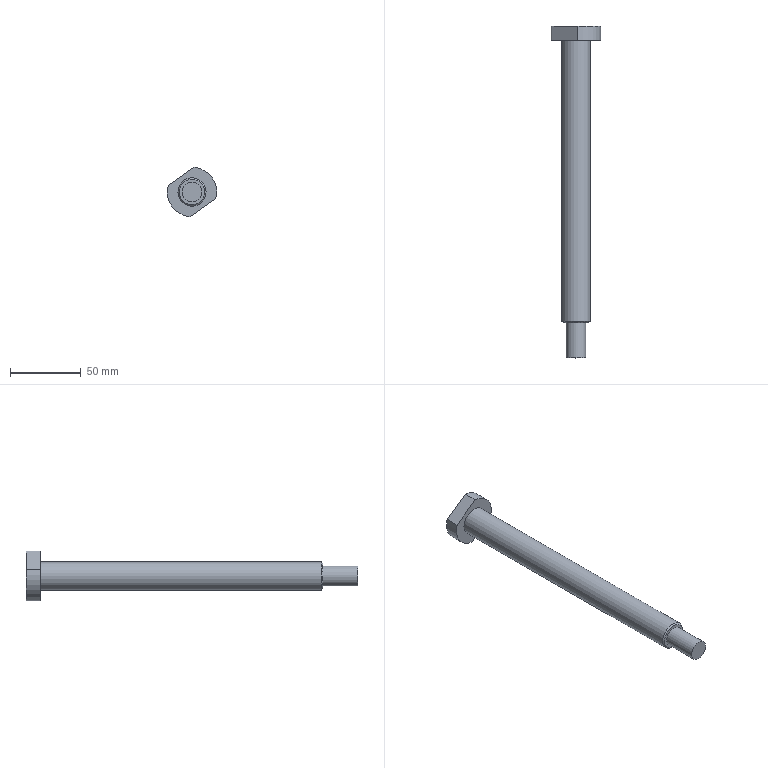Part | STEP file | HL4GZ-1.862.041 (cane-lifter mechanism mounting pin weldment) | 2 solids | 15 faces | box 35 x 235 x 34.891 mm | volume 74372 mm3 | plane 8 | cylinder 6 | cone 1 | commonest cylinder face diameters 17 x2 35 x2 14 x1 20 x1
STEP:
#1=CARTESIAN_POINT('',(0.,0.,0.));
#2=DIRECTION('',(0.,0.,1.));
#3=DIRECTION('',(1.,0.,0.));
#4=AXIS2_PLACEMENT_3D('',#1,#2,#3);
#5=CARTESIAN_POINT('',(3183.622,700.,-296.446));
#6=VERTEX_POINT('',#5);
#7=CARTESIAN_POINT('',(3183.622,690.,-296.446));
#8=VERTEX_POINT('',#7);
#9=CARTESIAN_POINT('',(3183.622,698.,-296.446));
#10=DIRECTION('',(0.,-1.,0.));
#11=VECTOR('',#10,1.);
#12=LINE('',#9,#11);
#13=CARTESIAN_POINT('',(3192.743,691.5,-290.059));
#14=DIRECTION('',(0.5736,0.,-0.8192));
#15=DIRECTION('',(0.8192,0.,0.5736));
#16=AXIS2_PLACEMENT_3D('',#13,#14,#15);
#17=PLANE('',#16);
#18=CARTESIAN_POINT('',(-11.136,-6.5));
#19=DIRECTION('',(0.,1.));
#20=VECTOR('',#19,1.);
#21=LINE('',#18,#20);
#22=(GEOMETRIC_REPRESENTATION_CONTEXT(2)PARAMETRIC_REPRESENTATION_CONTEXT()REPRESENTATION_CONTEXT('',''));
#23=DEFINITIONAL_REPRESENTATION('',(#21),#22);
#24=PCURVE('',#17,#23);
#25=CARTESIAN_POINT('',(3185.,690.,-279.));
#26=DIRECTION('',(0.,1.,0.));
#27=DIRECTION('',(0.06875,0.,0.9976));
#28=AXIS2_PLACEMENT_3D('',#25,#26,#27);
#29=CYLINDRICAL_SURFACE('',#28,17.5);
#30=CARTESIAN_POINT('',(3.152,8.));
#31=DIRECTION('',(0.,-1.));
#32=VECTOR('',#31,1.);
#33=LINE('',#30,#32);
#34=(GEOMETRIC_REPRESENTATION_CONTEXT(2)PARAMETRIC_REPRESENTATION_CONTEXT()REPRESENTATION_CONTEXT('',''));
#35=DEFINITIONAL_REPRESENTATION('',(#33),#34);
#36=PCURVE('',#29,#35);
#37=SURFACE_CURVE('',#12,(#24,#36),.PCURVE_S1.);
#38=EDGE_CURVE('',#6,#8,#37,.T.);
#39=ORIENTED_EDGE('',*,*,#38,.F.);
#40=CARTESIAN_POINT('',(3201.865,700.,-283.671));
#41=VERTEX_POINT('',#40);
#42=CARTESIAN_POINT('',(3192.743,700.,-290.059));
#43=DIRECTION('',(0.8192,0.,0.5736));
#44=VECTOR('',#43,1.);
#45=LINE('',#42,#44);
#46=CARTESIAN_POINT('',(0.,-8.5));
#47=DIRECTION('',(1.,0.));
#48=VECTOR('',#47,1.);
#49=LINE('',#46,#48);
#50=(GEOMETRIC_REPRESENTATION_CONTEXT(2)PARAMETRIC_REPRESENTATION_CONTEXT()REPRESENTATION_CONTEXT('',''));
#51=DEFINITIONAL_REPRESENTATION('',(#49),#50);
#52=PCURVE('',#17,#51);
#53=CARTESIAN_POINT('',(3184.927,700.,-278.896));
#54=DIRECTION('',(0.,-1.,0.));
#55=DIRECTION('',(0.8192,0.,0.5736));
#56=AXIS2_PLACEMENT_3D('',#53,#54,#55);
#57=PLANE('',#56);
#58=CARTESIAN_POINT('',(0.,-13.627));
#59=DIRECTION('',(1.,0.));
#60=VECTOR('',#59,1.);
#61=LINE('',#58,#60);
#62=(GEOMETRIC_REPRESENTATION_CONTEXT(2)PARAMETRIC_REPRESENTATION_CONTEXT()REPRESENTATION_CONTEXT('',''));
#63=DEFINITIONAL_REPRESENTATION('',(#61),#62);
#64=PCURVE('',#57,#63);
#65=SURFACE_CURVE('',#45,(#52,#64),.PCURVE_S1.);
#66=EDGE_CURVE('',#6,#41,#65,.T.);
#67=ORIENTED_EDGE('',*,*,#66,.T.);
#68=CARTESIAN_POINT('',(3201.865,690.,-283.671));
#69=VERTEX_POINT('',#68);
#70=CARTESIAN_POINT('',(3201.865,690.,-283.671));
#71=DIRECTION('',(0.,1.,0.));
#72=VECTOR('',#71,1.);
#73=LINE('',#70,#72);
#74=CARTESIAN_POINT('',(11.136,1.5));
#75=DIRECTION('',(0.,-1.));
#76=VECTOR('',#75,1.);
#77=LINE('',#74,#76);
#78=(GEOMETRIC_REPRESENTATION_CONTEXT(2)PARAMETRIC_REPRESENTATION_CONTEXT()REPRESENTATION_CONTEXT('',''));
#79=DEFINITIONAL_REPRESENTATION('',(#77),#78);
#80=PCURVE('',#17,#79);
#81=CARTESIAN_POINT('',(3185.,690.,-279.));
#82=DIRECTION('',(0.,1.,0.));
#83=DIRECTION('',(0.06875,0.,0.9976));
#84=AXIS2_PLACEMENT_3D('',#81,#82,#83);
#85=CYLINDRICAL_SURFACE('',#84,17.5);
#86=CARTESIAN_POINT('',(1.772,0.));
#87=DIRECTION('',(0.,1.));
#88=VECTOR('',#87,1.);
#89=LINE('',#86,#88);
#90=(GEOMETRIC_REPRESENTATION_CONTEXT(2)PARAMETRIC_REPRESENTATION_CONTEXT()REPRESENTATION_CONTEXT('',''));
#91=DEFINITIONAL_REPRESENTATION('',(#89),#90);
#92=PCURVE('',#85,#91);
#93=SURFACE_CURVE('',#73,(#80,#92),.PCURVE_S1.);
#94=EDGE_CURVE('',#69,#41,#93,.T.);
#95=ORIENTED_EDGE('',*,*,#94,.F.);
#96=CARTESIAN_POINT('',(3192.743,690.,-290.059));
#97=DIRECTION('',(0.8192,0.,0.5736));
#98=VECTOR('',#97,1.);
#99=LINE('',#96,#98);
#100=CARTESIAN_POINT('',(0.,1.5));
#101=DIRECTION('',(1.,0.));
#102=VECTOR('',#101,1.);
#103=LINE('',#100,#102);
#104=(GEOMETRIC_REPRESENTATION_CONTEXT(2)PARAMETRIC_REPRESENTATION_CONTEXT()REPRESENTATION_CONTEXT('',''));
#105=DEFINITIONAL_REPRESENTATION('',(#103),#104);
#106=PCURVE('',#17,#105);
#107=CARTESIAN_POINT('',(3184.927,690.,-278.896));
#108=DIRECTION('',(0.,-1.,0.));
#109=DIRECTION('',(0.8192,0.,0.5736));
#110=AXIS2_PLACEMENT_3D('',#107,#108,#109);
#111=PLANE('',#110);
#112=CARTESIAN_POINT('',(0.,-13.627));
#113=DIRECTION('',(1.,0.));
#114=VECTOR('',#113,1.);
#115=LINE('',#112,#114);
#116=(GEOMETRIC_REPRESENTATION_CONTEXT(2)PARAMETRIC_REPRESENTATION_CONTEXT()REPRESENTATION_CONTEXT('',''));
#117=DEFINITIONAL_REPRESENTATION('',(#115),#116);
#118=PCURVE('',#111,#117);
#119=SURFACE_CURVE('',#99,(#106,#118),.PCURVE_S1.);
#120=EDGE_CURVE('',#8,#69,#119,.T.);
#121=ORIENTED_EDGE('',*,*,#120,.F.);
#122=EDGE_LOOP('',(#39,#67,#95,#121));
#123=FACE_BOUND('',#122,.T.);
#124=ADVANCED_FACE('',(#123),#17,.T.);
#125=CARTESIAN_POINT('',(3168.135,690.,-274.328));
#126=VERTEX_POINT('',#125);
#127=CARTESIAN_POINT('',(3186.378,690.,-261.554));
#128=VERTEX_POINT('',#127);
#129=CARTESIAN_POINT('',(3167.989,690.,-274.431));
#130=DIRECTION('',(0.8192,0.,0.5736));
#131=VECTOR('',#130,1.);
#132=LINE('',#129,#131);
#133=CARTESIAN_POINT('',(3167.989,690.,-274.431));
#134=DIRECTION('',(-0.5736,0.,0.8192));
#135=DIRECTION('',(0.8192,0.,0.5736));
#136=AXIS2_PLACEMENT_3D('',#133,#134,#135);
#137=PLANE('',#136);
#138=CARTESIAN_POINT('',(0.,0.));
#139=DIRECTION('',(1.,0.));
#140=VECTOR('',#139,1.);
#141=LINE('',#138,#140);
#142=(GEOMETRIC_REPRESENTATION_CONTEXT(2)PARAMETRIC_REPRESENTATION_CONTEXT()REPRESENTATION_CONTEXT('',''));
#143=DEFINITIONAL_REPRESENTATION('',(#141),#142);
#144=PCURVE('',#137,#143);
#145=CARTESIAN_POINT('',(-11.314,13.373));
#146=DIRECTION('',(1.,0.));
#147=VECTOR('',#146,1.);
#148=LINE('',#145,#147);
#149=(GEOMETRIC_REPRESENTATION_CONTEXT(2)PARAMETRIC_REPRESENTATION_CONTEXT()REPRESENTATION_CONTEXT('',''));
#150=DEFINITIONAL_REPRESENTATION('',(#148),#149);
#151=PCURVE('',#111,#150);
#152=SURFACE_CURVE('',#132,(#144,#151),.PCURVE_S1.);
#153=EDGE_CURVE('',#126,#128,#152,.T.);
#154=ORIENTED_EDGE('',*,*,#153,.T.);
#155=CARTESIAN_POINT('',(3186.378,700.,-261.554));
#156=VERTEX_POINT('',#155);
#157=CARTESIAN_POINT('',(3186.378,690.,-261.554));
#158=DIRECTION('',(0.,1.,0.));
#159=VECTOR('',#158,1.);
#160=LINE('',#157,#159);
#161=CARTESIAN_POINT('',(22.449,0.));
#162=DIRECTION('',(0.,1.));
#163=VECTOR('',#162,1.);
#164=LINE('',#161,#163);
#165=(GEOMETRIC_REPRESENTATION_CONTEXT(2)PARAMETRIC_REPRESENTATION_CONTEXT()REPRESENTATION_CONTEXT('',''));
#166=DEFINITIONAL_REPRESENTATION('',(#164),#165);
#167=PCURVE('',#137,#166);
#168=CARTESIAN_POINT('',(0.01004,0.));
#169=DIRECTION('',(0.,1.));
#170=VECTOR('',#169,1.);
#171=LINE('',#168,#170);
#172=(GEOMETRIC_REPRESENTATION_CONTEXT(2)PARAMETRIC_REPRESENTATION_CONTEXT()REPRESENTATION_CONTEXT('',''));
#173=DEFINITIONAL_REPRESENTATION('',(#171),#172);
#174=PCURVE('',#85,#173);
#175=SURFACE_CURVE('',#160,(#167,#174),.PCURVE_S1.);
#176=EDGE_CURVE('',#128,#156,#175,.T.);
#177=ORIENTED_EDGE('',*,*,#176,.T.);
#178=CARTESIAN_POINT('',(3168.135,700.,-274.328));
#179=VERTEX_POINT('',#178);
#180=CARTESIAN_POINT('',(3167.989,700.,-274.431));
#181=DIRECTION('',(0.8192,0.,0.5736));
#182=VECTOR('',#181,1.);
#183=LINE('',#180,#182);
#184=CARTESIAN_POINT('',(0.,10.));
#185=DIRECTION('',(1.,0.));
#186=VECTOR('',#185,1.);
#187=LINE('',#184,#186);
#188=(GEOMETRIC_REPRESENTATION_CONTEXT(2)PARAMETRIC_REPRESENTATION_CONTEXT()REPRESENTATION_CONTEXT('',''));
#189=DEFINITIONAL_REPRESENTATION('',(#187),#188);
#190=PCURVE('',#137,#189);
#191=CARTESIAN_POINT('',(-11.314,13.373));
#192=DIRECTION('',(1.,0.));
#193=VECTOR('',#192,1.);
#194=LINE('',#191,#193);
#195=(GEOMETRIC_REPRESENTATION_CONTEXT(2)PARAMETRIC_REPRESENTATION_CONTEXT()REPRESENTATION_CONTEXT('',''));
#196=DEFINITIONAL_REPRESENTATION('',(#194),#195);
#197=PCURVE('',#57,#196);
#198=SURFACE_CURVE('',#183,(#190,#197),.PCURVE_S1.);
#199=EDGE_CURVE('',#179,#156,#198,.T.);
#200=ORIENTED_EDGE('',*,*,#199,.F.);
#201=CARTESIAN_POINT('',(3168.135,690.,-274.328));
#202=DIRECTION('',(0.,1.,0.));
#203=VECTOR('',#202,1.);
#204=LINE('',#201,#203);
#205=CARTESIAN_POINT('',(0.1782,0.));
#206=DIRECTION('',(0.,1.));
#207=VECTOR('',#206,1.);
#208=LINE('',#205,#207);
#209=(GEOMETRIC_REPRESENTATION_CONTEXT(2)PARAMETRIC_REPRESENTATION_CONTEXT()REPRESENTATION_CONTEXT('',''));
#210=DEFINITIONAL_REPRESENTATION('',(#208),#209);
#211=PCURVE('',#137,#210);
#212=CARTESIAN_POINT('',(4.914,0.));
#213=DIRECTION('',(0.,1.));
#214=VECTOR('',#213,1.);
#215=LINE('',#212,#214);
#216=(GEOMETRIC_REPRESENTATION_CONTEXT(2)PARAMETRIC_REPRESENTATION_CONTEXT()REPRESENTATION_CONTEXT('',''));
#217=DEFINITIONAL_REPRESENTATION('',(#215),#216);
#218=PCURVE('',#29,#217);
#219=SURFACE_CURVE('',#204,(#211,#218),.PCURVE_S1.);
#220=EDGE_CURVE('',#126,#179,#219,.T.);
#221=ORIENTED_EDGE('',*,*,#220,.F.);
#222=EDGE_LOOP('',(#154,#177,#200,#221));
#223=FACE_BOUND('',#222,.T.);
#224=ADVANCED_FACE('',(#223),#137,.T.);
#225=CARTESIAN_POINT('',(3185.,690.,-287.5));
#226=VERTEX_POINT('',#225);
#227=CARTESIAN_POINT('',(3185.,690.,-279.));
#228=DIRECTION('',(0.,1.,0.));
#229=DIRECTION('',(0.,0.,-1.));
#230=AXIS2_PLACEMENT_3D('',#227,#228,#229);
#231=CIRCLE('',#230,8.5);
#232=CARTESIAN_POINT('',(3185.,690.,-279.));
#233=DIRECTION('',(0.,1.,0.));
#234=DIRECTION('',(0.8192,0.,0.5736));
#235=AXIS2_PLACEMENT_3D('',#232,#233,#234);
#236=CYLINDRICAL_SURFACE('',#235,8.5);
#237=CARTESIAN_POINT('',(2.182,0.));
#238=DIRECTION('',(1.,0.));
#239=VECTOR('',#238,1.);
#240=LINE('',#237,#239);
#241=(GEOMETRIC_REPRESENTATION_CONTEXT(2)PARAMETRIC_REPRESENTATION_CONTEXT()REPRESENTATION_CONTEXT('',''));
#242=DEFINITIONAL_REPRESENTATION('',(#240),#241);
#243=PCURVE('',#236,#242);
#244=CARTESIAN_POINT('',(-4.875,-7.09));
#245=CARTESIAN_POINT('',(-16.935,1.355));
#246=CARTESIAN_POINT('',(-3.592,7.577));
#247=CARTESIAN_POINT('',(9.751,13.799));
#248=CARTESIAN_POINT('',(8.468,-0.8678));
#249=CARTESIAN_POINT('',(7.185,-15.534));
#250=CARTESIAN_POINT('',(-4.875,-7.09));
#251=(BOUNDED_CURVE()B_SPLINE_CURVE(2,(#244,#245,#246,#247,#248,#249,#250),.UNSPECIFIED.,.T.,.F.)B_SPLINE_CURVE_WITH_KNOTS((1,2,2,2,2,1),(-2.094,0.,2.094,4.189,6.283,8.378),.UNSPECIFIED.)CURVE()GEOMETRIC_REPRESENTATION_ITEM()RATIONAL_B_SPLINE_CURVE((1.,0.5,1.,0.5,1.,0.5,1.))REPRESENTATION_ITEM(''));
#252=(GEOMETRIC_REPRESENTATION_CONTEXT(2)PARAMETRIC_REPRESENTATION_CONTEXT()REPRESENTATION_CONTEXT('',''));
#253=DEFINITIONAL_REPRESENTATION('',(#251),#252);
#254=PCURVE('',#111,#253);
#255=SURFACE_CURVE('',#231,(#243,#254),.PCURVE_S1.);
#256=EDGE_CURVE('',#226,#226,#255,.T.);
#257=ORIENTED_EDGE('',*,*,#256,.T.);
#258=CARTESIAN_POINT('',(3185.,700.,-287.5));
#259=VERTEX_POINT('',#258);
#260=CARTESIAN_POINT('',(3185.,690.,-287.5));
#261=CARTESIAN_POINT('',(3185.,700.,-287.5));
#262=B_SPLINE_CURVE_WITH_KNOTS('',1,(#260,#261),.UNSPECIFIED.,.F.,.F.,(2,2),(0.,10.),.PIECEWISE_BEZIER_KNOTS.);
#263=CARTESIAN_POINT('',(8.465,0.));
#264=DIRECTION('',(0.,1.));
#265=VECTOR('',#264,1.);
#266=LINE('',#263,#265);
#267=(GEOMETRIC_REPRESENTATION_CONTEXT(2)PARAMETRIC_REPRESENTATION_CONTEXT()REPRESENTATION_CONTEXT('',''));
#268=DEFINITIONAL_REPRESENTATION('',(#266),#267);
#269=PCURVE('',#236,#268);
#270=CARTESIAN_POINT('',(2.182,0.));
#271=DIRECTION('',(0.,1.));
#272=VECTOR('',#271,1.);
#273=LINE('',#270,#272);
#274=(GEOMETRIC_REPRESENTATION_CONTEXT(2)PARAMETRIC_REPRESENTATION_CONTEXT()REPRESENTATION_CONTEXT('',''));
#275=DEFINITIONAL_REPRESENTATION('',(#273),#274);
#276=PCURVE('',#236,#275);
#277=SEAM_CURVE('',#262,(#269,#276),.PCURVE_S1.);
#278=EDGE_CURVE('',#226,#259,#277,.T.);
#279=ORIENTED_EDGE('',*,*,#278,.T.);
#280=CARTESIAN_POINT('',(3185.,700.,-279.));
#281=DIRECTION('',(0.,-1.,0.));
#282=DIRECTION('',(0.,0.,-1.));
#283=AXIS2_PLACEMENT_3D('',#280,#281,#282);
#284=CIRCLE('',#283,8.5);
#285=CARTESIAN_POINT('',(8.465,10.));
#286=DIRECTION('',(-1.,0.));
#287=VECTOR('',#286,1.);
#288=LINE('',#285,#287);
#289=(GEOMETRIC_REPRESENTATION_CONTEXT(2)PARAMETRIC_REPRESENTATION_CONTEXT()REPRESENTATION_CONTEXT('',''));
#290=DEFINITIONAL_REPRESENTATION('',(#288),#289);
#291=PCURVE('',#236,#290);
#292=CARTESIAN_POINT('',(0.,-0.127));
#293=DIRECTION('',(-0.5736,-0.8192));
#294=AXIS2_PLACEMENT_2D('',#292,#293);
#295=CIRCLE('',#294,8.5);
#296=(GEOMETRIC_REPRESENTATION_CONTEXT(2)PARAMETRIC_REPRESENTATION_CONTEXT()REPRESENTATION_CONTEXT('',''));
#297=DEFINITIONAL_REPRESENTATION('',(#295),#296);
#298=PCURVE('',#57,#297);
#299=SURFACE_CURVE('',#284,(#291,#298),.PCURVE_S1.);
#300=EDGE_CURVE('',#259,#259,#299,.T.);
#301=ORIENTED_EDGE('',*,*,#300,.T.);
#302=ORIENTED_EDGE('',*,*,#278,.F.);
#303=EDGE_LOOP('',(#257,#279,#301,#302));
#304=FACE_BOUND('',#303,.F.);
#305=ADVANCED_FACE('',(#304),#236,.F.);
#306=CARTESIAN_POINT('',(3185.,690.,-279.));
#307=DIRECTION('',(0.,1.,0.));
#308=DIRECTION('',(0.,0.,-1.));
#309=AXIS2_PLACEMENT_3D('',#306,#307,#308);
#310=CIRCLE('',#309,17.5);
#311=CARTESIAN_POINT('',(-10.038,-14.462));
#312=CARTESIAN_POINT('',(-34.867,2.923));
#313=CARTESIAN_POINT('',(-7.396,15.733));
#314=CARTESIAN_POINT('',(20.075,28.543));
#315=CARTESIAN_POINT('',(17.433,-1.652));
#316=CARTESIAN_POINT('',(14.792,-31.848));
#317=CARTESIAN_POINT('',(-10.038,-14.462));
#318=(BOUNDED_CURVE()B_SPLINE_CURVE(2,(#311,#312,#313,#314,#315,#316,#317),.UNSPECIFIED.,.T.,.F.)B_SPLINE_CURVE_WITH_KNOTS((1,2,2,2,2,1),(-2.094,0.,2.094,4.189,6.283,8.378),.UNSPECIFIED.)CURVE()GEOMETRIC_REPRESENTATION_ITEM()RATIONAL_B_SPLINE_CURVE((1.,0.5,1.,0.5,1.,0.5,1.))REPRESENTATION_ITEM(''));
#319=(GEOMETRIC_REPRESENTATION_CONTEXT(2)PARAMETRIC_REPRESENTATION_CONTEXT()REPRESENTATION_CONTEXT('',''));
#320=DEFINITIONAL_REPRESENTATION('',(#318),#319);
#321=PCURVE('',#111,#320);
#322=CARTESIAN_POINT('',(3.073,0.));
#323=DIRECTION('',(1.,0.));
#324=VECTOR('',#323,1.);
#325=LINE('',#322,#324);
#326=(GEOMETRIC_REPRESENTATION_CONTEXT(2)PARAMETRIC_REPRESENTATION_CONTEXT()REPRESENTATION_CONTEXT('',''));
#327=DEFINITIONAL_REPRESENTATION('',(#325),#326);
#328=PCURVE('',#29,#327);
#329=SURFACE_CURVE('',#310,(#321,#328),.PCURVE_S1.);
#330=EDGE_CURVE('',#8,#126,#329,.T.);
#331=ORIENTED_EDGE('',*,*,#330,.F.);
#332=ORIENTED_EDGE('',*,*,#120,.T.);
#333=CARTESIAN_POINT('',(3185.,690.,-279.));
#334=DIRECTION('',(0.,1.,0.));
#335=DIRECTION('',(0.,0.,-1.));
#336=AXIS2_PLACEMENT_3D('',#333,#334,#335);
#337=CIRCLE('',#336,17.5);
#338=CARTESIAN_POINT('',(-10.038,-14.462));
#339=CARTESIAN_POINT('',(-34.867,2.923));
#340=CARTESIAN_POINT('',(-7.396,15.733));
#341=CARTESIAN_POINT('',(20.075,28.543));
#342=CARTESIAN_POINT('',(17.433,-1.652));
#343=CARTESIAN_POINT('',(14.792,-31.848));
#344=CARTESIAN_POINT('',(-10.038,-14.462));
#345=(BOUNDED_CURVE()B_SPLINE_CURVE(2,(#338,#339,#340,#341,#342,#343,#344),.UNSPECIFIED.,.T.,.F.)B_SPLINE_CURVE_WITH_KNOTS((1,2,2,2,2,1),(-2.094,0.,2.094,4.189,6.283,8.378),.UNSPECIFIED.)CURVE()GEOMETRIC_REPRESENTATION_ITEM()RATIONAL_B_SPLINE_CURVE((1.,0.5,1.,0.5,1.,0.5,1.))REPRESENTATION_ITEM(''));
#346=(GEOMETRIC_REPRESENTATION_CONTEXT(2)PARAMETRIC_REPRESENTATION_CONTEXT()REPRESENTATION_CONTEXT('',''));
#347=DEFINITIONAL_REPRESENTATION('',(#345),#346);
#348=PCURVE('',#111,#347);
#349=CARTESIAN_POINT('',(-3.21,0.));
#350=DIRECTION('',(1.,0.));
#351=VECTOR('',#350,1.);
#352=LINE('',#349,#351);
#353=(GEOMETRIC_REPRESENTATION_CONTEXT(2)PARAMETRIC_REPRESENTATION_CONTEXT()REPRESENTATION_CONTEXT('',''));
#354=DEFINITIONAL_REPRESENTATION('',(#352),#353);
#355=PCURVE('',#85,#354);
#356=SURFACE_CURVE('',#337,(#348,#355),.PCURVE_S1.);
#357=EDGE_CURVE('',#128,#69,#356,.T.);
#358=ORIENTED_EDGE('',*,*,#357,.F.);
#359=ORIENTED_EDGE('',*,*,#153,.F.);
#360=EDGE_LOOP('',(#331,#332,#358,#359));
#361=FACE_BOUND('',#360,.T.);
#362=ORIENTED_EDGE('',*,*,#256,.T.);
#363=EDGE_LOOP('',(#362));
#364=FACE_BOUND('',#363,.T.);
#365=ADVANCED_FACE('',(#361,#364),#111,.T.);
#366=ORIENTED_EDGE('',*,*,#66,.F.);
#367=CARTESIAN_POINT('',(3185.,700.,-279.));
#368=DIRECTION('',(0.,1.,0.));
#369=DIRECTION('',(0.,0.,-1.));
#370=AXIS2_PLACEMENT_3D('',#367,#368,#369);
#371=CIRCLE('',#370,17.5);
#372=CARTESIAN_POINT('',(-10.038,-14.462));
#373=CARTESIAN_POINT('',(-34.867,2.923));
#374=CARTESIAN_POINT('',(-7.396,15.733));
#375=CARTESIAN_POINT('',(20.075,28.543));
#376=CARTESIAN_POINT('',(17.433,-1.652));
#377=CARTESIAN_POINT('',(14.792,-31.848));
#378=CARTESIAN_POINT('',(-10.038,-14.462));
#379=(BOUNDED_CURVE()B_SPLINE_CURVE(2,(#372,#373,#374,#375,#376,#377,#378),.UNSPECIFIED.,.T.,.F.)B_SPLINE_CURVE_WITH_KNOTS((1,2,2,2,2,1),(-2.094,0.,2.094,4.189,6.283,8.378),.UNSPECIFIED.)CURVE()GEOMETRIC_REPRESENTATION_ITEM()RATIONAL_B_SPLINE_CURVE((1.,0.5,1.,0.5,1.,0.5,1.))REPRESENTATION_ITEM(''));
#380=(GEOMETRIC_REPRESENTATION_CONTEXT(2)PARAMETRIC_REPRESENTATION_CONTEXT()REPRESENTATION_CONTEXT('',''));
#381=DEFINITIONAL_REPRESENTATION('',(#379),#380);
#382=PCURVE('',#57,#381);
#383=CARTESIAN_POINT('',(3.073,10.));
#384=DIRECTION('',(1.,0.));
#385=VECTOR('',#384,1.);
#386=LINE('',#383,#385);
#387=(GEOMETRIC_REPRESENTATION_CONTEXT(2)PARAMETRIC_REPRESENTATION_CONTEXT()REPRESENTATION_CONTEXT('',''));
#388=DEFINITIONAL_REPRESENTATION('',(#386),#387);
#389=PCURVE('',#29,#388);
#390=SURFACE_CURVE('',#371,(#382,#389),.PCURVE_S1.);
#391=EDGE_CURVE('',#6,#179,#390,.T.);
#392=ORIENTED_EDGE('',*,*,#391,.T.);
#393=ORIENTED_EDGE('',*,*,#199,.T.);
#394=CARTESIAN_POINT('',(3185.,700.,-279.));
#395=DIRECTION('',(0.,1.,0.));
#396=DIRECTION('',(0.,0.,-1.));
#397=AXIS2_PLACEMENT_3D('',#394,#395,#396);
#398=CIRCLE('',#397,17.5);
#399=CARTESIAN_POINT('',(-10.038,-14.462));
#400=CARTESIAN_POINT('',(-34.867,2.923));
#401=CARTESIAN_POINT('',(-7.396,15.733));
#402=CARTESIAN_POINT('',(20.075,28.543));
#403=CARTESIAN_POINT('',(17.433,-1.652));
#404=CARTESIAN_POINT('',(14.792,-31.848));
#405=CARTESIAN_POINT('',(-10.038,-14.462));
#406=(BOUNDED_CURVE()B_SPLINE_CURVE(2,(#399,#400,#401,#402,#403,#404,#405),.UNSPECIFIED.,.T.,.F.)B_SPLINE_CURVE_WITH_KNOTS((1,2,2,2,2,1),(-2.094,0.,2.094,4.189,6.283,8.378),.UNSPECIFIED.)CURVE()GEOMETRIC_REPRESENTATION_ITEM()RATIONAL_B_SPLINE_CURVE((1.,0.5,1.,0.5,1.,0.5,1.))REPRESENTATION_ITEM(''));
#407=(GEOMETRIC_REPRESENTATION_CONTEXT(2)PARAMETRIC_REPRESENTATION_CONTEXT()REPRESENTATION_CONTEXT('',''));
#408=DEFINITIONAL_REPRESENTATION('',(#406),#407);
#409=PCURVE('',#57,#408);
#410=CARTESIAN_POINT('',(-3.21,10.));
#411=DIRECTION('',(1.,0.));
#412=VECTOR('',#411,1.);
#413=LINE('',#410,#412);
#414=(GEOMETRIC_REPRESENTATION_CONTEXT(2)PARAMETRIC_REPRESENTATION_CONTEXT()REPRESENTATION_CONTEXT('',''));
#415=DEFINITIONAL_REPRESENTATION('',(#413),#414);
#416=PCURVE('',#85,#415);
#417=SURFACE_CURVE('',#398,(#409,#416),.PCURVE_S1.);
#418=EDGE_CURVE('',#156,#41,#417,.T.);
#419=ORIENTED_EDGE('',*,*,#418,.T.);
#420=EDGE_LOOP('',(#366,#392,#393,#419));
#421=FACE_BOUND('',#420,.T.);
#422=ORIENTED_EDGE('',*,*,#300,.T.);
#423=EDGE_LOOP('',(#422));
#424=FACE_BOUND('',#423,.T.);
#425=ADVANCED_FACE('',(#421,#424),#57,.F.);
#426=ORIENTED_EDGE('',*,*,#357,.T.);
#427=ORIENTED_EDGE('',*,*,#94,.T.);
#428=ORIENTED_EDGE('',*,*,#418,.F.);
#429=ORIENTED_EDGE('',*,*,#176,.F.);
#430=EDGE_LOOP('',(#426,#427,#428,#429));
#431=FACE_BOUND('',#430,.T.);
#432=ADVANCED_FACE('',(#431),#85,.T.);
#433=ORIENTED_EDGE('',*,*,#391,.F.);
#434=ORIENTED_EDGE('',*,*,#38,.T.);
#435=ORIENTED_EDGE('',*,*,#330,.T.);
#436=ORIENTED_EDGE('',*,*,#220,.T.);
#437=EDGE_LOOP('',(#433,#434,#435,#436));
#438=FACE_BOUND('',#437,.T.);
#439=ADVANCED_FACE('',(#438),#29,.T.);
#440=CLOSED_SHELL('',(#124,#224,#305,#365,#425,#432,#439));
#441=MANIFOLD_SOLID_BREP('',#440);
#442=CARTESIAN_POINT('',(3185.,490.,-286.));
#443=VERTEX_POINT('',#442);
#444=CARTESIAN_POINT('',(3185.,490.,-279.));
#445=DIRECTION('',(0.,-1.,0.));
#446=DIRECTION('',(0.,0.,-1.));
#447=AXIS2_PLACEMENT_3D('',#444,#445,#446);
#448=CIRCLE('',#447,7.);
#449=CARTESIAN_POINT('',(3185.,477.,-279.));
#450=DIRECTION('',(0.,-1.,0.));
#451=DIRECTION('',(0.5736,0.,-0.8192));
#452=AXIS2_PLACEMENT_3D('',#449,#450,#451);
#453=CYLINDRICAL_SURFACE('',#452,7.);
#454=CARTESIAN_POINT('',(5.672,-13.));
#455=DIRECTION('',(1.,0.));
#456=VECTOR('',#455,1.);
#457=LINE('',#454,#456);
#458=(GEOMETRIC_REPRESENTATION_CONTEXT(2)PARAMETRIC_REPRESENTATION_CONTEXT()REPRESENTATION_CONTEXT('',''));
#459=DEFINITIONAL_REPRESENTATION('',(#457),#458);
#460=PCURVE('',#453,#459);
#461=CARTESIAN_POINT('',(3188.441,490.,-283.915));
#462=DIRECTION('',(0.,-1.,0.));
#463=DIRECTION('',(-0.8192,0.,-0.5736));
#464=AXIS2_PLACEMENT_3D('',#461,#462,#463);
#465=PLANE('',#464);
#466=CARTESIAN_POINT('',(0.,-6.));
#467=DIRECTION('',(0.5736,0.8192));
#468=AXIS2_PLACEMENT_2D('',#466,#467);
#469=CIRCLE('',#468,7.);
#470=(GEOMETRIC_REPRESENTATION_CONTEXT(2)PARAMETRIC_REPRESENTATION_CONTEXT()REPRESENTATION_CONTEXT('',''));
#471=DEFINITIONAL_REPRESENTATION('',(#469),#470);
#472=PCURVE('',#465,#471);
#473=SURFACE_CURVE('',#448,(#460,#472),.PCURVE_S1.);
#474=EDGE_CURVE('',#443,#443,#473,.T.);
#475=ORIENTED_EDGE('',*,*,#474,.T.);
#476=CARTESIAN_POINT('',(3185.,465.,-286.));
#477=VERTEX_POINT('',#476);
#478=CARTESIAN_POINT('',(3185.,490.,-286.));
#479=CARTESIAN_POINT('',(3185.,465.,-286.));
#480=B_SPLINE_CURVE_WITH_KNOTS('',1,(#478,#479),.UNSPECIFIED.,.F.,.F.,(2,2),(-13.,12.),.PIECEWISE_BEZIER_KNOTS.);
#481=CARTESIAN_POINT('',(11.956,0.));
#482=DIRECTION('',(0.,1.));
#483=VECTOR('',#482,1.);
#484=LINE('',#481,#483);
#485=(GEOMETRIC_REPRESENTATION_CONTEXT(2)PARAMETRIC_REPRESENTATION_CONTEXT()REPRESENTATION_CONTEXT('',''));
#486=DEFINITIONAL_REPRESENTATION('',(#484),#485);
#487=PCURVE('',#453,#486);
#488=CARTESIAN_POINT('',(5.672,0.));
#489=DIRECTION('',(0.,1.));
#490=VECTOR('',#489,1.);
#491=LINE('',#488,#490);
#492=(GEOMETRIC_REPRESENTATION_CONTEXT(2)PARAMETRIC_REPRESENTATION_CONTEXT()REPRESENTATION_CONTEXT('',''));
#493=DEFINITIONAL_REPRESENTATION('',(#491),#492);
#494=PCURVE('',#453,#493);
#495=SEAM_CURVE('',#480,(#487,#494),.PCURVE_S1.);
#496=EDGE_CURVE('',#443,#477,#495,.T.);
#497=ORIENTED_EDGE('',*,*,#496,.T.);
#498=CARTESIAN_POINT('',(3185.,465.,-279.));
#499=DIRECTION('',(0.,-1.,0.));
#500=DIRECTION('',(0.,0.,-1.));
#501=AXIS2_PLACEMENT_3D('',#498,#499,#500);
#502=CIRCLE('',#501,7.);
#503=CARTESIAN_POINT('',(5.672,12.));
#504=DIRECTION('',(1.,0.));
#505=VECTOR('',#504,1.);
#506=LINE('',#503,#505);
#507=(GEOMETRIC_REPRESENTATION_CONTEXT(2)PARAMETRIC_REPRESENTATION_CONTEXT()REPRESENTATION_CONTEXT('',''));
#508=DEFINITIONAL_REPRESENTATION('',(#506),#507);
#509=PCURVE('',#453,#508);
#510=CARTESIAN_POINT('',(3185.,465.,-279.));
#511=DIRECTION('',(0.,-1.,0.));
#512=DIRECTION('',(-0.8192,0.,-0.5736));
#513=AXIS2_PLACEMENT_3D('',#510,#511,#512);
#514=PLANE('',#513);
#515=CARTESIAN_POINT('',(0.,0.));
#516=DIRECTION('',(0.5736,0.8192));
#517=AXIS2_PLACEMENT_2D('',#515,#516);
#518=CIRCLE('',#517,7.);
#519=(GEOMETRIC_REPRESENTATION_CONTEXT(2)PARAMETRIC_REPRESENTATION_CONTEXT()REPRESENTATION_CONTEXT('',''));
#520=DEFINITIONAL_REPRESENTATION('',(#518),#519);
#521=PCURVE('',#514,#520);
#522=SURFACE_CURVE('',#502,(#509,#521),.PCURVE_S1.);
#523=EDGE_CURVE('',#477,#477,#522,.T.);
#524=ORIENTED_EDGE('',*,*,#523,.F.);
#525=ORIENTED_EDGE('',*,*,#496,.F.);
#526=EDGE_LOOP('',(#475,#497,#524,#525));
#527=FACE_BOUND('',#526,.T.);
#528=ADVANCED_FACE('',(#527),#453,.T.);
#529=CARTESIAN_POINT('',(3185.,690.,-270.5));
#530=VERTEX_POINT('',#529);
#531=CARTESIAN_POINT('',(3185.,690.,-287.5));
#532=VERTEX_POINT('',#531);
#533=CARTESIAN_POINT('',(3185.,690.,-279.));
#534=DIRECTION('',(0.,-1.,0.));
#535=DIRECTION('',(0.,0.,1.));
#536=AXIS2_PLACEMENT_3D('',#533,#534,#535);
#537=CIRCLE('',#536,8.5);
#538=CARTESIAN_POINT('',(3190.736,690.,-287.191));
#539=DIRECTION('',(0.,1.,0.));
#540=DIRECTION('',(0.8192,0.,0.5736));
#541=AXIS2_PLACEMENT_3D('',#538,#539,#540);
#542=PLANE('',#541);
#543=CARTESIAN_POINT('',(4.875,-16.963));
#544=CARTESIAN_POINT('',(-7.185,-25.407));
#545=CARTESIAN_POINT('',(-8.468,-10.741));
#546=CARTESIAN_POINT('',(-9.751,3.926));
#547=CARTESIAN_POINT('',(3.592,-2.296));
#548=CARTESIAN_POINT('',(16.935,-8.518));
#549=CARTESIAN_POINT('',(4.875,-16.963));
#550=(BOUNDED_CURVE()B_SPLINE_CURVE(2,(#543,#544,#545,#546,#547,#548,#549),.UNSPECIFIED.,.T.,.F.)B_SPLINE_CURVE_WITH_KNOTS((1,2,2,2,2,1),(-2.094,0.,2.094,4.189,6.283,8.378),.UNSPECIFIED.)CURVE()GEOMETRIC_REPRESENTATION_ITEM()RATIONAL_B_SPLINE_CURVE((1.,0.5,1.,0.5,1.,0.5,1.))REPRESENTATION_ITEM(''));
#551=(GEOMETRIC_REPRESENTATION_CONTEXT(2)PARAMETRIC_REPRESENTATION_CONTEXT()REPRESENTATION_CONTEXT('',''));
#552=DEFINITIONAL_REPRESENTATION('',(#550),#551);
#553=PCURVE('',#542,#552);
#554=CARTESIAN_POINT('',(3185.,690.,-279.));
#555=DIRECTION('',(0.,1.,0.));
#556=DIRECTION('',(-0.8192,0.,-0.5736));
#557=AXIS2_PLACEMENT_3D('',#554,#555,#556);
#558=CYLINDRICAL_SURFACE('',#557,8.5);
#559=CARTESIAN_POINT('',(8.465,0.));
#560=DIRECTION('',(-1.,0.));
#561=VECTOR('',#560,1.);
#562=LINE('',#559,#561);
#563=(GEOMETRIC_REPRESENTATION_CONTEXT(2)PARAMETRIC_REPRESENTATION_CONTEXT()REPRESENTATION_CONTEXT('',''));
#564=DEFINITIONAL_REPRESENTATION('',(#562),#563);
#565=PCURVE('',#558,#564);
#566=SURFACE_CURVE('',#537,(#553,#565),.PCURVE_S1.);
#567=EDGE_CURVE('',#530,#532,#566,.T.);
#568=ORIENTED_EDGE('',*,*,#567,.T.);
#569=CARTESIAN_POINT('',(3185.,690.,-279.));
#570=DIRECTION('',(0.,-1.,0.));
#571=DIRECTION('',(0.,0.,1.));
#572=AXIS2_PLACEMENT_3D('',#569,#570,#571);
#573=CIRCLE('',#572,8.5);
#574=CARTESIAN_POINT('',(4.875,-16.963));
#575=CARTESIAN_POINT('',(-7.185,-25.407));
#576=CARTESIAN_POINT('',(-8.468,-10.741));
#577=CARTESIAN_POINT('',(-9.751,3.926));
#578=CARTESIAN_POINT('',(3.592,-2.296));
#579=CARTESIAN_POINT('',(16.935,-8.518));
#580=CARTESIAN_POINT('',(4.875,-16.963));
#581=(BOUNDED_CURVE()B_SPLINE_CURVE(2,(#574,#575,#576,#577,#578,#579,#580),.UNSPECIFIED.,.T.,.F.)B_SPLINE_CURVE_WITH_KNOTS((1,2,2,2,2,1),(-2.094,0.,2.094,4.189,6.283,8.378),.UNSPECIFIED.)CURVE()GEOMETRIC_REPRESENTATION_ITEM()RATIONAL_B_SPLINE_CURVE((1.,0.5,1.,0.5,1.,0.5,1.))REPRESENTATION_ITEM(''));
#582=(GEOMETRIC_REPRESENTATION_CONTEXT(2)PARAMETRIC_REPRESENTATION_CONTEXT()REPRESENTATION_CONTEXT('',''));
#583=DEFINITIONAL_REPRESENTATION('',(#581),#582);
#584=PCURVE('',#542,#583);
#585=CARTESIAN_POINT('',(14.748,0.));
#586=DIRECTION('',(-1.,0.));
#587=VECTOR('',#586,1.);
#588=LINE('',#585,#587);
#589=(GEOMETRIC_REPRESENTATION_CONTEXT(2)PARAMETRIC_REPRESENTATION_CONTEXT()REPRESENTATION_CONTEXT('',''));
#590=DEFINITIONAL_REPRESENTATION('',(#588),#589);
#591=PCURVE('',#558,#590);
#592=SURFACE_CURVE('',#573,(#584,#591),.PCURVE_S1.);
#593=EDGE_CURVE('',#532,#530,#592,.T.);
#594=ORIENTED_EDGE('',*,*,#593,.T.);
#595=EDGE_LOOP('',(#568,#594));
#596=FACE_BOUND('',#595,.T.);
#597=CARTESIAN_POINT('',(3190.736,690.,-287.191));
#598=VERTEX_POINT('',#597);
#599=CARTESIAN_POINT('',(3185.,690.,-279.));
#600=DIRECTION('',(0.,-1.,0.));
#601=DIRECTION('',(-0.8192,0.,-0.5736));
#602=AXIS2_PLACEMENT_3D('',#599,#600,#601);
#603=CIRCLE('',#602,10.);
#604=CARTESIAN_POINT('',(-10.,-10.));
#605=CARTESIAN_POINT('',(-10.,7.321));
#606=CARTESIAN_POINT('',(5.,-1.34));
#607=CARTESIAN_POINT('',(20.,-10.));
#608=CARTESIAN_POINT('',(5.,-18.66));
#609=CARTESIAN_POINT('',(-10.,-27.321));
#610=CARTESIAN_POINT('',(-10.,-10.));
#611=(BOUNDED_CURVE()B_SPLINE_CURVE(2,(#604,#605,#606,#607,#608,#609,#610),.UNSPECIFIED.,.T.,.F.)B_SPLINE_CURVE_WITH_KNOTS((1,2,2,2,2,1),(-2.094,0.,2.094,4.189,6.283,8.378),.UNSPECIFIED.)CURVE()GEOMETRIC_REPRESENTATION_ITEM()RATIONAL_B_SPLINE_CURVE((1.,0.5,1.,0.5,1.,0.5,1.))REPRESENTATION_ITEM(''));
#612=(GEOMETRIC_REPRESENTATION_CONTEXT(2)PARAMETRIC_REPRESENTATION_CONTEXT()REPRESENTATION_CONTEXT('',''));
#613=DEFINITIONAL_REPRESENTATION('',(#611),#612);
#614=PCURVE('',#542,#613);
#615=CARTESIAN_POINT('',(3185.,590.,-279.));
#616=DIRECTION('',(0.,-1.,0.));
#617=DIRECTION('',(0.5736,0.,-0.8192));
#618=AXIS2_PLACEMENT_3D('',#615,#616,#617);
#619=CYLINDRICAL_SURFACE('',#618,10.);
#620=CARTESIAN_POINT('',(-1.571,-100.));
#621=DIRECTION('',(1.,0.));
#622=VECTOR('',#621,1.);
#623=LINE('',#620,#622);
#624=(GEOMETRIC_REPRESENTATION_CONTEXT(2)PARAMETRIC_REPRESENTATION_CONTEXT()REPRESENTATION_CONTEXT('',''));
#625=DEFINITIONAL_REPRESENTATION('',(#623),#624);
#626=PCURVE('',#619,#625);
#627=SURFACE_CURVE('',#603,(#614,#626),.PCURVE_S1.);
#628=EDGE_CURVE('',#598,#598,#627,.T.);
#629=ORIENTED_EDGE('',*,*,#628,.F.);
#630=EDGE_LOOP('',(#629));
#631=FACE_BOUND('',#630,.T.);
#632=ADVANCED_FACE('',(#596,#631),#542,.T.);
#633=CARTESIAN_POINT('',(3185.,697.,-287.5));
#634=VERTEX_POINT('',#633);
#635=CARTESIAN_POINT('',(3185.,697.,-279.));
#636=DIRECTION('',(0.,1.,0.));
#637=DIRECTION('',(0.,0.,-1.));
#638=AXIS2_PLACEMENT_3D('',#635,#636,#637);
#639=CIRCLE('',#638,8.5);
#640=CARTESIAN_POINT('',(3185.,697.,-279.));
#641=DIRECTION('',(0.,-1.,0.));
#642=DIRECTION('',(-0.8192,0.,-0.5736));
#643=AXIS2_PLACEMENT_3D('',#640,#641,#642);
#644=PLANE('',#643);
#645=CARTESIAN_POINT('',(4.875,6.963));
#646=CARTESIAN_POINT('',(16.935,-1.482));
#647=CARTESIAN_POINT('',(3.592,-7.704));
#648=CARTESIAN_POINT('',(-9.751,-13.926));
#649=CARTESIAN_POINT('',(-8.468,0.7408));
#650=CARTESIAN_POINT('',(-7.185,15.407));
#651=CARTESIAN_POINT('',(4.875,6.963));
#652=(BOUNDED_CURVE()B_SPLINE_CURVE(2,(#645,#646,#647,#648,#649,#650,#651),.UNSPECIFIED.,.T.,.F.)B_SPLINE_CURVE_WITH_KNOTS((1,2,2,2,2,1),(-2.094,0.,2.094,4.189,6.283,8.378),.UNSPECIFIED.)CURVE()GEOMETRIC_REPRESENTATION_ITEM()RATIONAL_B_SPLINE_CURVE((1.,0.5,1.,0.5,1.,0.5,1.))REPRESENTATION_ITEM(''));
#653=(GEOMETRIC_REPRESENTATION_CONTEXT(2)PARAMETRIC_REPRESENTATION_CONTEXT()REPRESENTATION_CONTEXT('',''));
#654=DEFINITIONAL_REPRESENTATION('',(#652),#653);
#655=PCURVE('',#644,#654);
#656=CARTESIAN_POINT('',(5.323,7.));
#657=DIRECTION('',(1.,0.));
#658=VECTOR('',#657,1.);
#659=LINE('',#656,#658);
#660=(GEOMETRIC_REPRESENTATION_CONTEXT(2)PARAMETRIC_REPRESENTATION_CONTEXT()REPRESENTATION_CONTEXT('',''));
#661=DEFINITIONAL_REPRESENTATION('',(#659),#660);
#662=PCURVE('',#558,#661);
#663=SURFACE_CURVE('',#639,(#655,#662),.PCURVE_S1.);
#664=EDGE_CURVE('',#634,#634,#663,.T.);
#665=ORIENTED_EDGE('',*,*,#664,.T.);
#666=EDGE_LOOP('',(#665));
#667=FACE_BOUND('',#666,.T.);
#668=ADVANCED_FACE('',(#667),#644,.F.);
#669=ORIENTED_EDGE('',*,*,#593,.F.);
#670=CARTESIAN_POINT('',(3185.,690.,-287.5));
#671=CARTESIAN_POINT('',(3185.,697.,-287.5));
#672=B_SPLINE_CURVE_WITH_KNOTS('',1,(#670,#671),.UNSPECIFIED.,.F.,.F.,(2,2),(0.,7.),.PIECEWISE_BEZIER_KNOTS.);
#673=CARTESIAN_POINT('',(11.606,0.));
#674=DIRECTION('',(0.,1.));
#675=VECTOR('',#674,1.);
#676=LINE('',#673,#675);
#677=(GEOMETRIC_REPRESENTATION_CONTEXT(2)PARAMETRIC_REPRESENTATION_CONTEXT()REPRESENTATION_CONTEXT('',''));
#678=DEFINITIONAL_REPRESENTATION('',(#676),#677);
#679=PCURVE('',#558,#678);
#680=CARTESIAN_POINT('',(5.323,0.));
#681=DIRECTION('',(0.,1.));
#682=VECTOR('',#681,1.);
#683=LINE('',#680,#682);
#684=(GEOMETRIC_REPRESENTATION_CONTEXT(2)PARAMETRIC_REPRESENTATION_CONTEXT()REPRESENTATION_CONTEXT('',''));
#685=DEFINITIONAL_REPRESENTATION('',(#683),#684);
#686=PCURVE('',#558,#685);
#687=SEAM_CURVE('',#672,(#679,#686),.PCURVE_S1.);
#688=EDGE_CURVE('',#532,#634,#687,.T.);
#689=ORIENTED_EDGE('',*,*,#688,.T.);
#690=ORIENTED_EDGE('',*,*,#664,.F.);
#691=ORIENTED_EDGE('',*,*,#688,.F.);
#692=ORIENTED_EDGE('',*,*,#567,.F.);
#693=EDGE_LOOP('',(#669,#689,#690,#691,#692));
#694=FACE_BOUND('',#693,.T.);
#695=ADVANCED_FACE('',(#694),#558,.T.);
#696=CARTESIAN_POINT('',(3190.162,490.,-286.372));
#697=VERTEX_POINT('',#696);
#698=CARTESIAN_POINT('',(3185.,490.,-279.));
#699=DIRECTION('',(0.,1.,0.));
#700=DIRECTION('',(-0.5736,0.,0.8192));
#701=AXIS2_PLACEMENT_3D('',#698,#699,#700);
#702=CIRCLE('',#701,9.);
#703=CARTESIAN_POINT('',(0.,-15.));
#704=CARTESIAN_POINT('',(-15.588,-15.));
#705=CARTESIAN_POINT('',(-7.794,-1.5));
#706=CARTESIAN_POINT('',(0.,12.));
#707=CARTESIAN_POINT('',(7.794,-1.5));
#708=CARTESIAN_POINT('',(15.588,-15.));
#709=CARTESIAN_POINT('',(0.,-15.));
#710=(BOUNDED_CURVE()B_SPLINE_CURVE(2,(#703,#704,#705,#706,#707,#708,#709),.UNSPECIFIED.,.T.,.F.)B_SPLINE_CURVE_WITH_KNOTS((1,2,2,2,2,1),(-2.094,0.,2.094,4.189,6.283,8.378),.UNSPECIFIED.)CURVE()GEOMETRIC_REPRESENTATION_ITEM()RATIONAL_B_SPLINE_CURVE((1.,0.5,1.,0.5,1.,0.5,1.))REPRESENTATION_ITEM(''));
#711=(GEOMETRIC_REPRESENTATION_CONTEXT(2)PARAMETRIC_REPRESENTATION_CONTEXT()REPRESENTATION_CONTEXT('',''));
#712=DEFINITIONAL_REPRESENTATION('',(#710),#711);
#713=PCURVE('',#465,#712);
#714=CARTESIAN_POINT('',(3185.,490.5,-279.));
#715=DIRECTION('',(0.,1.,0.));
#716=DIRECTION('',(-0.5736,0.,0.8192));
#717=AXIS2_PLACEMENT_3D('',#714,#715,#716);
#718=CONICAL_SURFACE('',#717,9.5,0.7854);
#719=CARTESIAN_POINT('',(0.,-0.5));
#720=DIRECTION('',(1.,0.));
#721=VECTOR('',#720,1.);
#722=LINE('',#719,#721);
#723=(GEOMETRIC_REPRESENTATION_CONTEXT(2)PARAMETRIC_REPRESENTATION_CONTEXT()REPRESENTATION_CONTEXT('',''));
#724=DEFINITIONAL_REPRESENTATION('',(#722),#723);
#725=PCURVE('',#718,#724);
#726=SURFACE_CURVE('',#702,(#713,#725),.PCURVE_S1.);
#727=EDGE_CURVE('',#697,#697,#726,.T.);
#728=ORIENTED_EDGE('',*,*,#727,.F.);
#729=EDGE_LOOP('',(#728));
#730=FACE_BOUND('',#729,.T.);
#731=ORIENTED_EDGE('',*,*,#474,.F.);
#732=EDGE_LOOP('',(#731));
#733=FACE_BOUND('',#732,.T.);
#734=ADVANCED_FACE('',(#730,#733),#465,.T.);
#735=CARTESIAN_POINT('',(3190.736,491.,-287.191));
#736=VERTEX_POINT('',#735);
#737=CARTESIAN_POINT('',(3185.,491.,-279.));
#738=DIRECTION('',(0.,-1.,0.));
#739=DIRECTION('',(-0.5736,0.,0.8192));
#740=AXIS2_PLACEMENT_3D('',#737,#738,#739);
#741=CIRCLE('',#740,10.);
#742=CARTESIAN_POINT('',(-3.142,99.));
#743=DIRECTION('',(1.,0.));
#744=VECTOR('',#743,1.);
#745=LINE('',#742,#744);
#746=(GEOMETRIC_REPRESENTATION_CONTEXT(2)PARAMETRIC_REPRESENTATION_CONTEXT()REPRESENTATION_CONTEXT('',''));
#747=DEFINITIONAL_REPRESENTATION('',(#745),#746);
#748=PCURVE('',#619,#747);
#749=CARTESIAN_POINT('',(12.566,0.5));
#750=DIRECTION('',(-1.,0.));
#751=VECTOR('',#750,1.);
#752=LINE('',#749,#751);
#753=(GEOMETRIC_REPRESENTATION_CONTEXT(2)PARAMETRIC_REPRESENTATION_CONTEXT()REPRESENTATION_CONTEXT('',''));
#754=DEFINITIONAL_REPRESENTATION('',(#752),#753);
#755=PCURVE('',#718,#754);
#756=SURFACE_CURVE('',#741,(#748,#755),.PCURVE_S1.);
#757=EDGE_CURVE('',#736,#736,#756,.T.);
#758=ORIENTED_EDGE('',*,*,#757,.F.);
#759=CARTESIAN_POINT('',(3190.736,690.,-287.191));
#760=CARTESIAN_POINT('',(3190.736,491.,-287.191));
#761=B_SPLINE_CURVE_WITH_KNOTS('',1,(#759,#760),.UNSPECIFIED.,.F.,.F.,(2,2),(-100.,99.),.PIECEWISE_BEZIER_KNOTS.);
#762=CARTESIAN_POINT('',(0.,0.));
#763=DIRECTION('',(0.,1.));
#764=VECTOR('',#763,1.);
#765=LINE('',#762,#764);
#766=(GEOMETRIC_REPRESENTATION_CONTEXT(2)PARAMETRIC_REPRESENTATION_CONTEXT()REPRESENTATION_CONTEXT('',''));
#767=DEFINITIONAL_REPRESENTATION('',(#765),#766);
#768=PCURVE('',#619,#767);
#769=CARTESIAN_POINT('',(6.283,0.));
#770=DIRECTION('',(0.,1.));
#771=VECTOR('',#770,1.);
#772=LINE('',#769,#771);
#773=(GEOMETRIC_REPRESENTATION_CONTEXT(2)PARAMETRIC_REPRESENTATION_CONTEXT()REPRESENTATION_CONTEXT('',''));
#774=DEFINITIONAL_REPRESENTATION('',(#772),#773);
#775=PCURVE('',#619,#774);
#776=SEAM_CURVE('',#761,(#768,#775),.PCURVE_S1.);
#777=EDGE_CURVE('',#598,#736,#776,.T.);
#778=ORIENTED_EDGE('',*,*,#777,.F.);
#779=ORIENTED_EDGE('',*,*,#628,.T.);
#780=ORIENTED_EDGE('',*,*,#777,.T.);
#781=EDGE_LOOP('',(#758,#778,#779,#780));
#782=FACE_BOUND('',#781,.T.);
#783=ADVANCED_FACE('',(#782),#619,.T.);
#784=ORIENTED_EDGE('',*,*,#727,.T.);
#785=CARTESIAN_POINT('',(3190.162,490.,-286.372));
#786=CARTESIAN_POINT('',(3190.736,491.,-287.191));
#787=B_SPLINE_CURVE_WITH_KNOTS('',1,(#785,#786),.UNSPECIFIED.,.F.,.F.,(2,2),(-0.7071,0.7071),.PIECEWISE_BEZIER_KNOTS.);
#788=CARTESIAN_POINT('',(9.425,0.));
#789=DIRECTION('',(0.,1.));
#790=VECTOR('',#789,1.);
#791=LINE('',#788,#790);
#792=(GEOMETRIC_REPRESENTATION_CONTEXT(2)PARAMETRIC_REPRESENTATION_CONTEXT()REPRESENTATION_CONTEXT('',''));
#793=DEFINITIONAL_REPRESENTATION('',(#791),#792);
#794=PCURVE('',#718,#793);
#795=CARTESIAN_POINT('',(3.142,0.));
#796=DIRECTION('',(0.,1.));
#797=VECTOR('',#796,1.);
#798=LINE('',#795,#797);
#799=(GEOMETRIC_REPRESENTATION_CONTEXT(2)PARAMETRIC_REPRESENTATION_CONTEXT()REPRESENTATION_CONTEXT('',''));
#800=DEFINITIONAL_REPRESENTATION('',(#798),#799);
#801=PCURVE('',#718,#800);
#802=SEAM_CURVE('',#787,(#794,#801),.PCURVE_S1.);
#803=EDGE_CURVE('',#697,#736,#802,.T.);
#804=ORIENTED_EDGE('',*,*,#803,.T.);
#805=ORIENTED_EDGE('',*,*,#757,.T.);
#806=ORIENTED_EDGE('',*,*,#803,.F.);
#807=EDGE_LOOP('',(#784,#804,#805,#806));
#808=FACE_BOUND('',#807,.T.);
#809=ADVANCED_FACE('',(#808),#718,.T.);
#810=ORIENTED_EDGE('',*,*,#523,.T.);
#811=EDGE_LOOP('',(#810));
#812=FACE_BOUND('',#811,.T.);
#813=ADVANCED_FACE('',(#812),#514,.T.);
#814=CLOSED_SHELL('',(#528,#632,#668,#695,#734,#783,#809,#813));
#815=MANIFOLD_SOLID_BREP('',#814);
#816=(LENGTH_UNIT()NAMED_UNIT(*)SI_UNIT(.MILLI.,.METRE.));
#817=UNCERTAINTY_MEASURE_WITH_UNIT(LENGTH_MEASURE(0.000005),#816,'','');
#818=(NAMED_UNIT(*)PLANE_ANGLE_UNIT()SI_UNIT($,.RADIAN.));
#819=(NAMED_UNIT(*)SI_UNIT($,.STERADIAN.)SOLID_ANGLE_UNIT());
#820=(GEOMETRIC_REPRESENTATION_CONTEXT(3)GLOBAL_UNCERTAINTY_ASSIGNED_CONTEXT((#817))GLOBAL_UNIT_ASSIGNED_CONTEXT((#816,#818,#819))REPRESENTATION_CONTEXT('',''));
#821=SHAPE_REPRESENTATION('',(#4,#441,#815),#820);